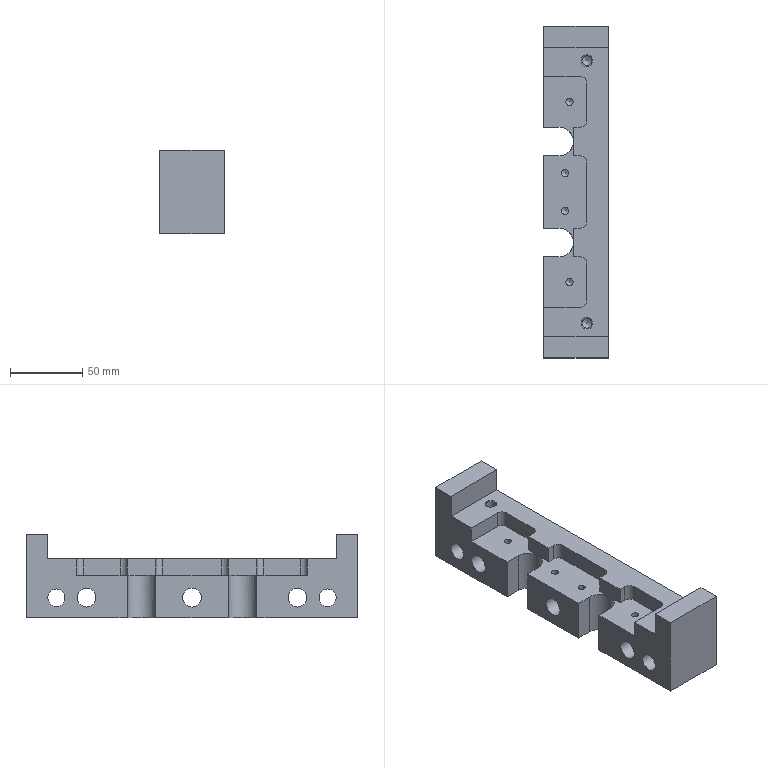Part | STEP file | lll_id354_x_t | 1 solid | 63 faces | box 45 x 230 x 58 mm | volume 337405 mm3 | plane 33 | cylinder 22 | cone 8 | commonest cylinder face diameters 9 x6 20 x5 5 x4 13 x3 6.8 x2 12 x2